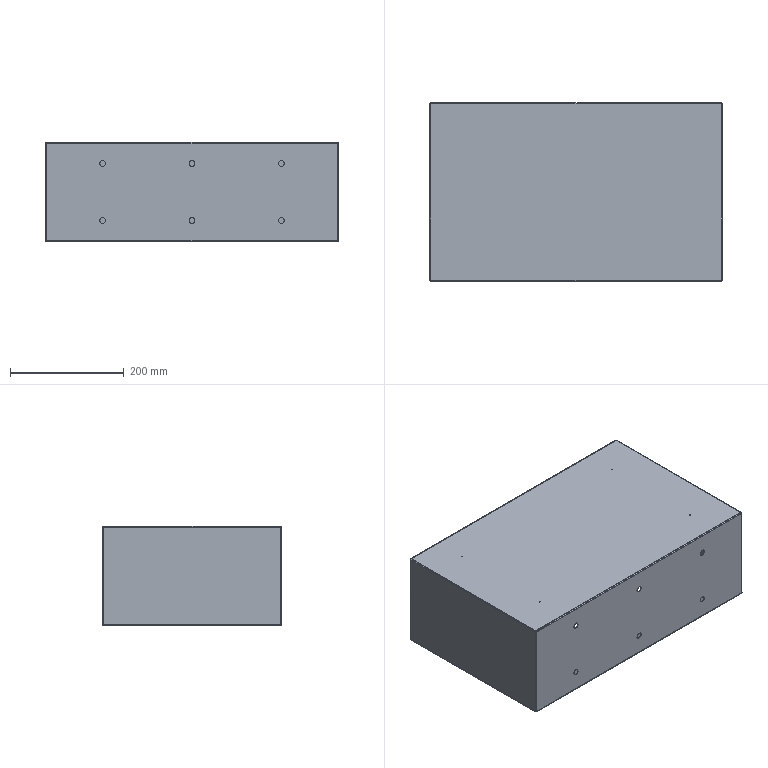Part | 1 solid | 190 faces | box 515 x 315 x 175 mm | volume 628618 mm3 | cylinder 80 | plane 78 | spline 32 | commonest cylinder face diameters 1.473 x16 3.873 x16 7 x16 10 x12 16 x12 2 x8